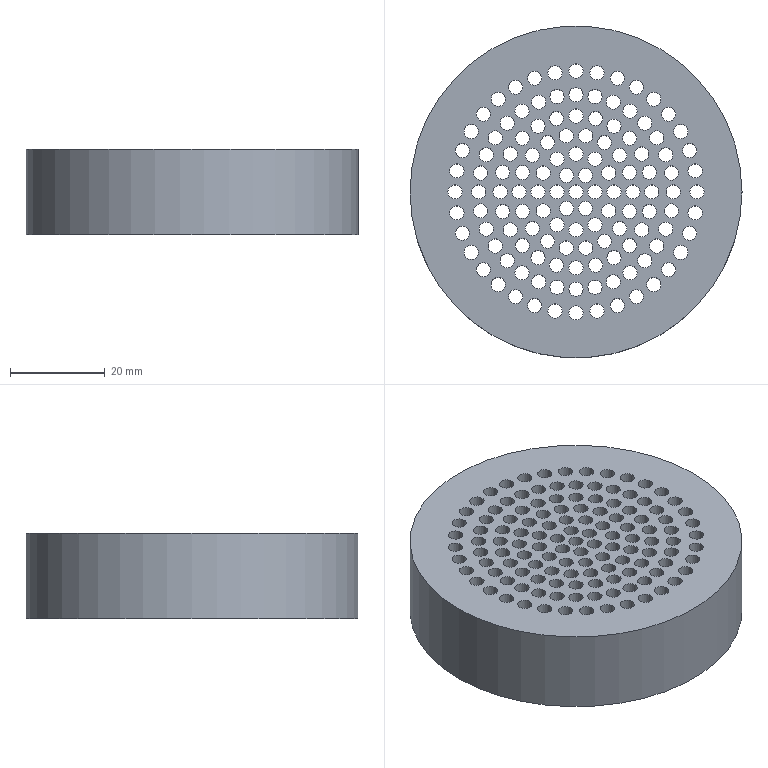Part | 1 solid | 132 faces | box 70 x 70 x 18 mm | volume 52859 mm3 | cylinder 130 | plane 2 | commonest cylinder face diameters 3 x129 70 x1